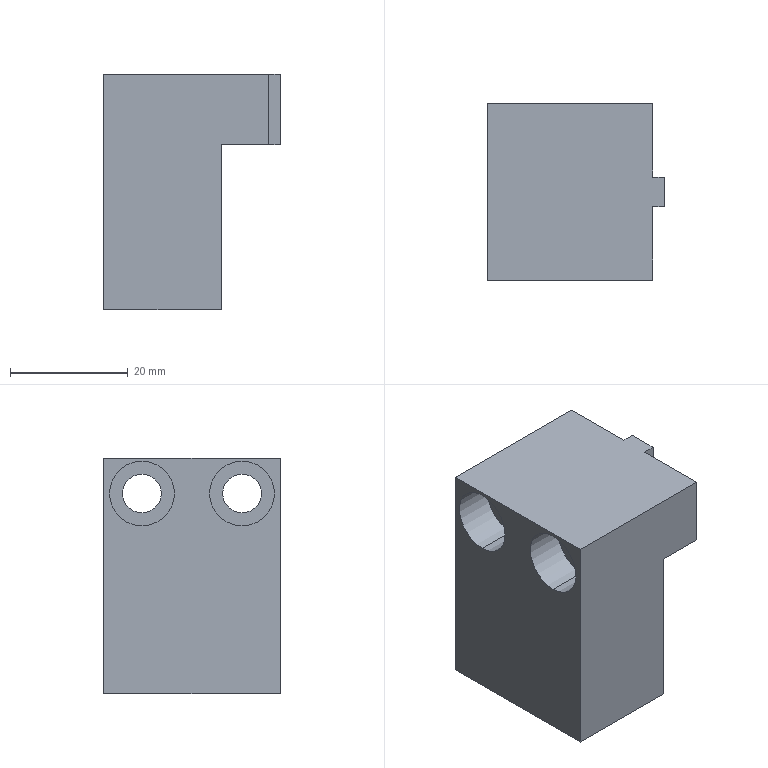Part | SolidWorks | features BaseBody 1 | 1 solid | 22 faces | box 30 x 30 x 40 mm | volume 24257 mm3 | plane 14 | cylinder 8 | commonest cylinder face diameters 6.6 x4 11 x4
STEP:
#1=CARTESIAN_POINT('',(-13.2,23.5,-11.5));
#2=VERTEX_POINT('',#1);
#3=CARTESIAN_POINT('',(-20.,23.5,-11.5));
#4=VERTEX_POINT('',#3);
#5=CARTESIAN_POINT('',(-20.,23.5,-11.5));
#6=DIRECTION('',(-1.,0.,0.));
#7=VECTOR('',#6,1000.);
#8=LINE('',#5,#7);
#9=EDGE_CURVE('',#2,#4,#8,.T.);
#10=ORIENTED_EDGE('',*,*,#9,.F.);
#11=CARTESIAN_POINT('',(-13.2,23.5,-0.5));
#12=VERTEX_POINT('',#11);
#13=CARTESIAN_POINT('',(-13.2,23.5,-6.));
#14=DIRECTION('',(-1.,0.,0.));
#15=DIRECTION('',(0.,0.,1.));
#16=AXIS2_PLACEMENT_3D('',#13,#14,#15);
#17=CIRCLE('',#16,5.5);
#18=EDGE_CURVE('',#12,#2,#17,.T.);
#19=ORIENTED_EDGE('',*,*,#18,.F.);
#20=CARTESIAN_POINT('',(-20.,23.5,-0.5));
#21=VERTEX_POINT('',#20);
#22=CARTESIAN_POINT('',(-20.,23.5,-0.5));
#23=DIRECTION('',(-1.,0.,0.));
#24=VECTOR('',#23,1000.);
#25=LINE('',#22,#24);
#26=EDGE_CURVE('',#12,#21,#25,.T.);
#27=ORIENTED_EDGE('',*,*,#26,.T.);
#28=CARTESIAN_POINT('',(-20.,23.5,-6.));
#29=DIRECTION('',(-1.,0.,0.));
#30=DIRECTION('',(0.,0.,1.));
#31=AXIS2_PLACEMENT_3D('',#28,#29,#30);
#32=CIRCLE('',#31,5.5);
#33=EDGE_CURVE('',#21,#4,#32,.T.);
#34=ORIENTED_EDGE('',*,*,#33,.T.);
#35=EDGE_LOOP('',(#10,#19,#27,#34));
#36=FACE_OUTER_BOUND('',#35,.T.);
#37=CARTESIAN_POINT('',(-20.,23.5,-6.));
#38=DIRECTION('',(-1.,0.,0.));
#39=DIRECTION('',(0.,0.,1.));
#40=AXIS2_PLACEMENT_3D('',#37,#38,#39);
#41=CYLINDRICAL_SURFACE('',#40,5.5);
#42=ADVANCED_FACE('',(#36),#41,.F.);
#43=CARTESIAN_POINT('',(-13.2,23.5,-2.7));
#44=VERTEX_POINT('',#43);
#45=CARTESIAN_POINT('',(-13.2,23.5,-9.3));
#46=VERTEX_POINT('',#45);
#47=CARTESIAN_POINT('',(-13.2,23.5,-6.));
#48=DIRECTION('',(-1.,0.,0.));
#49=DIRECTION('',(0.,0.,1.));
#50=AXIS2_PLACEMENT_3D('',#47,#48,#49);
#51=CIRCLE('',#50,3.3);
#52=EDGE_CURVE('',#44,#46,#51,.T.);
#53=ORIENTED_EDGE('',*,*,#52,.F.);
#54=CARTESIAN_POINT('',(-13.2,23.5,-6.));
#55=DIRECTION('',(-1.,0.,0.));
#56=DIRECTION('',(0.,0.,1.));
#57=AXIS2_PLACEMENT_3D('',#54,#55,#56);
#58=CIRCLE('',#57,3.3);
#59=EDGE_CURVE('',#46,#44,#58,.T.);
#60=ORIENTED_EDGE('',*,*,#59,.F.);
#61=EDGE_LOOP('',(#53,#60));
#62=FACE_BOUND('',#61,.T.);
#63=ORIENTED_EDGE('',*,*,#18,.T.);
#64=CARTESIAN_POINT('',(-13.2,23.5,-6.));
#65=DIRECTION('',(-1.,0.,0.));
#66=DIRECTION('',(0.,0.,1.));
#67=AXIS2_PLACEMENT_3D('',#64,#65,#66);
#68=CIRCLE('',#67,5.5);
#69=EDGE_CURVE('',#2,#12,#68,.T.);
#70=ORIENTED_EDGE('',*,*,#69,.T.);
#71=EDGE_LOOP('',(#63,#70));
#72=FACE_OUTER_BOUND('',#71,.T.);
#73=CARTESIAN_POINT('',(-13.2,26.8,-6.));
#74=DIRECTION('',(1.,0.,0.));
#75=DIRECTION('',(0.,0.,-1.));
#76=AXIS2_PLACEMENT_3D('',#73,#74,#75);
#77=PLANE('',#76);
#78=ADVANCED_FACE('',(#62,#72),#77,.F.);
#79=CARTESIAN_POINT('',(8.,23.5,-9.3));
#80=VERTEX_POINT('',#79);
#81=CARTESIAN_POINT('',(-20.,23.5,-9.3));
#82=DIRECTION('',(-1.,0.,0.));
#83=VECTOR('',#82,1000.);
#84=LINE('',#81,#83);
#85=EDGE_CURVE('',#80,#46,#84,.T.);
#86=ORIENTED_EDGE('',*,*,#85,.F.);
#87=CARTESIAN_POINT('',(8.,23.5,-2.7));
#88=VERTEX_POINT('',#87);
#89=CARTESIAN_POINT('',(8.,23.5,-6.));
#90=DIRECTION('',(1.,0.,0.));
#91=DIRECTION('',(0.,0.,-1.));
#92=AXIS2_PLACEMENT_3D('',#89,#90,#91);
#93=CIRCLE('',#92,3.3);
#94=EDGE_CURVE('',#80,#88,#93,.T.);
#95=ORIENTED_EDGE('',*,*,#94,.T.);
#96=CARTESIAN_POINT('',(-20.,23.5,-2.7));
#97=DIRECTION('',(-1.,0.,0.));
#98=VECTOR('',#97,1000.);
#99=LINE('',#96,#98);
#100=EDGE_CURVE('',#88,#44,#99,.T.);
#101=ORIENTED_EDGE('',*,*,#100,.T.);
#102=ORIENTED_EDGE('',*,*,#52,.T.);
#103=EDGE_LOOP('',(#86,#95,#101,#102));
#104=FACE_OUTER_BOUND('',#103,.T.);
#105=CARTESIAN_POINT('',(-20.,23.5,-6.));
#106=DIRECTION('',(-1.,0.,0.));
#107=DIRECTION('',(0.,0.,1.));
#108=AXIS2_PLACEMENT_3D('',#105,#106,#107);
#109=CYLINDRICAL_SURFACE('',#108,3.3);
#110=ADVANCED_FACE('',(#104),#109,.F.);
#111=CARTESIAN_POINT('',(-13.2,6.5,-11.5));
#112=VERTEX_POINT('',#111);
#113=CARTESIAN_POINT('',(-20.,6.5,-11.5));
#114=VERTEX_POINT('',#113);
#115=CARTESIAN_POINT('',(-20.,6.5,-11.5));
#116=DIRECTION('',(-1.,0.,0.));
#117=VECTOR('',#116,1000.);
#118=LINE('',#115,#117);
#119=EDGE_CURVE('',#112,#114,#118,.T.);
#120=ORIENTED_EDGE('',*,*,#119,.F.);
#121=CARTESIAN_POINT('',(-13.2,6.5,-0.5));
#122=VERTEX_POINT('',#121);
#123=CARTESIAN_POINT('',(-13.2,6.5,-6.));
#124=DIRECTION('',(-1.,0.,0.));
#125=DIRECTION('',(0.,0.,1.));
#126=AXIS2_PLACEMENT_3D('',#123,#124,#125);
#127=CIRCLE('',#126,5.5);
#128=EDGE_CURVE('',#122,#112,#127,.T.);
#129=ORIENTED_EDGE('',*,*,#128,.F.);
#130=CARTESIAN_POINT('',(-20.,6.5,-0.5));
#131=VERTEX_POINT('',#130);
#132=CARTESIAN_POINT('',(-20.,6.5,-0.5));
#133=DIRECTION('',(-1.,0.,0.));
#134=VECTOR('',#133,1000.);
#135=LINE('',#132,#134);
#136=EDGE_CURVE('',#122,#131,#135,.T.);
#137=ORIENTED_EDGE('',*,*,#136,.T.);
#138=CARTESIAN_POINT('',(-20.,6.5,-6.));
#139=DIRECTION('',(-1.,0.,0.));
#140=DIRECTION('',(0.,0.,1.));
#141=AXIS2_PLACEMENT_3D('',#138,#139,#140);
#142=CIRCLE('',#141,5.5);
#143=EDGE_CURVE('',#131,#114,#142,.T.);
#144=ORIENTED_EDGE('',*,*,#143,.T.);
#145=EDGE_LOOP('',(#120,#129,#137,#144));
#146=FACE_OUTER_BOUND('',#145,.T.);
#147=CARTESIAN_POINT('',(-20.,6.5,-6.));
#148=DIRECTION('',(-1.,0.,0.));
#149=DIRECTION('',(0.,0.,1.));
#150=AXIS2_PLACEMENT_3D('',#147,#148,#149);
#151=CYLINDRICAL_SURFACE('',#150,5.5);
#152=ADVANCED_FACE('',(#146),#151,.F.);
#153=CARTESIAN_POINT('',(-13.2,6.5,-2.7));
#154=VERTEX_POINT('',#153);
#155=CARTESIAN_POINT('',(-13.2,6.5,-9.3));
#156=VERTEX_POINT('',#155);
#157=CARTESIAN_POINT('',(-13.2,6.5,-6.));
#158=DIRECTION('',(-1.,0.,0.));
#159=DIRECTION('',(0.,0.,1.));
#160=AXIS2_PLACEMENT_3D('',#157,#158,#159);
#161=CIRCLE('',#160,3.3);
#162=EDGE_CURVE('',#154,#156,#161,.T.);
#163=ORIENTED_EDGE('',*,*,#162,.F.);
#164=CARTESIAN_POINT('',(-13.2,6.5,-6.));
#165=DIRECTION('',(-1.,0.,0.));
#166=DIRECTION('',(0.,0.,1.));
#167=AXIS2_PLACEMENT_3D('',#164,#165,#166);
#168=CIRCLE('',#167,3.3);
#169=EDGE_CURVE('',#156,#154,#168,.T.);
#170=ORIENTED_EDGE('',*,*,#169,.F.);
#171=EDGE_LOOP('',(#163,#170));
#172=FACE_BOUND('',#171,.T.);
#173=ORIENTED_EDGE('',*,*,#128,.T.);
#174=CARTESIAN_POINT('',(-13.2,6.5,-6.));
#175=DIRECTION('',(-1.,0.,0.));
#176=DIRECTION('',(0.,0.,1.));
#177=AXIS2_PLACEMENT_3D('',#174,#175,#176);
#178=CIRCLE('',#177,5.5);
#179=EDGE_CURVE('',#112,#122,#178,.T.);
#180=ORIENTED_EDGE('',*,*,#179,.T.);
#181=EDGE_LOOP('',(#173,#180));
#182=FACE_OUTER_BOUND('',#181,.T.);
#183=CARTESIAN_POINT('',(-13.2,9.8,-6.));
#184=DIRECTION('',(1.,0.,0.));
#185=DIRECTION('',(0.,0.,-1.));
#186=AXIS2_PLACEMENT_3D('',#183,#184,#185);
#187=PLANE('',#186);
#188=ADVANCED_FACE('',(#172,#182),#187,.F.);
#189=CARTESIAN_POINT('',(8.,6.5,-9.3));
#190=VERTEX_POINT('',#189);
#191=CARTESIAN_POINT('',(-20.,6.5,-9.3));
#192=DIRECTION('',(-1.,0.,0.));
#193=VECTOR('',#192,1000.);
#194=LINE('',#191,#193);
#195=EDGE_CURVE('',#190,#156,#194,.T.);
#196=ORIENTED_EDGE('',*,*,#195,.F.);
#197=CARTESIAN_POINT('',(8.,6.5,-2.7));
#198=VERTEX_POINT('',#197);
#199=CARTESIAN_POINT('',(8.,6.5,-6.));
#200=DIRECTION('',(1.,0.,0.));
#201=DIRECTION('',(0.,0.,-1.));
#202=AXIS2_PLACEMENT_3D('',#199,#200,#201);
#203=CIRCLE('',#202,3.3);
#204=EDGE_CURVE('',#190,#198,#203,.T.);
#205=ORIENTED_EDGE('',*,*,#204,.T.);
#206=CARTESIAN_POINT('',(-20.,6.5,-2.7));
#207=DIRECTION('',(-1.,0.,0.));
#208=VECTOR('',#207,1000.);
#209=LINE('',#206,#208);
#210=EDGE_CURVE('',#198,#154,#209,.T.);
#211=ORIENTED_EDGE('',*,*,#210,.T.);
#212=ORIENTED_EDGE('',*,*,#162,.T.);
#213=EDGE_LOOP('',(#196,#205,#211,#212));
#214=FACE_OUTER_BOUND('',#213,.T.);
#215=CARTESIAN_POINT('',(-20.,6.5,-6.));
#216=DIRECTION('',(-1.,0.,0.));
#217=DIRECTION('',(0.,0.,1.));
#218=AXIS2_PLACEMENT_3D('',#215,#216,#217);
#219=CYLINDRICAL_SURFACE('',#218,3.3);
#220=ADVANCED_FACE('',(#214),#219,.F.);
#221=CARTESIAN_POINT('',(8.,23.5,-6.));
#222=DIRECTION('',(1.,0.,0.));
#223=DIRECTION('',(0.,0.,-1.));
#224=AXIS2_PLACEMENT_3D('',#221,#222,#223);
#225=CIRCLE('',#224,3.3);
#226=EDGE_CURVE('',#88,#80,#225,.T.);
#227=ORIENTED_EDGE('',*,*,#226,.F.);
#228=ORIENTED_EDGE('',*,*,#94,.F.);
#229=EDGE_LOOP('',(#227,#228));
#230=FACE_BOUND('',#229,.T.);
#231=CARTESIAN_POINT('',(8.,30.,0.));
#232=VERTEX_POINT('',#231);
#233=CARTESIAN_POINT('',(8.,17.5,0.));
#234=VERTEX_POINT('',#233);
#235=CARTESIAN_POINT('',(8.,30.,0.));
#236=DIRECTION('',(0.,-1.,0.));
#237=VECTOR('',#236,1000.);
#238=LINE('',#235,#237);
#239=EDGE_CURVE('',#232,#234,#238,.T.);
#240=ORIENTED_EDGE('',*,*,#239,.T.);
#241=CARTESIAN_POINT('',(8.,17.5,-12.));
#242=VERTEX_POINT('',#241);
#243=CARTESIAN_POINT('',(8.,17.5,0.));
#244=DIRECTION('',(0.,0.,-1.));
#245=VECTOR('',#244,1000.);
#246=LINE('',#243,#245);
#247=EDGE_CURVE('',#234,#242,#246,.T.);
#248=ORIENTED_EDGE('',*,*,#247,.T.);
#249=CARTESIAN_POINT('',(8.,30.,-12.));
#250=VERTEX_POINT('',#249);
#251=CARTESIAN_POINT('',(8.,30.,-12.));
#252=DIRECTION('',(0.,1.,0.));
#253=VECTOR('',#252,1000.);
#254=LINE('',#251,#253);
#255=EDGE_CURVE('',#242,#250,#254,.T.);
#256=ORIENTED_EDGE('',*,*,#255,.T.);
#257=CARTESIAN_POINT('',(8.,30.,0.));
#258=DIRECTION('',(0.,0.,1.));
#259=VECTOR('',#258,1000.);
#260=LINE('',#257,#259);
#261=EDGE_CURVE('',#250,#232,#260,.T.);
#262=ORIENTED_EDGE('',*,*,#261,.T.);
#263=EDGE_LOOP('',(#240,#248,#256,#262));
#264=FACE_OUTER_BOUND('',#263,.T.);
#265=CARTESIAN_POINT('',(8.,0.,0.));
#266=DIRECTION('',(1.,0.,0.));
#267=DIRECTION('',(0.,1.,0.));
#268=AXIS2_PLACEMENT_3D('',#265,#266,#267);
#269=PLANE('',#268);
#270=ADVANCED_FACE('',(#230,#264),#269,.T.);
#271=CARTESIAN_POINT('',(10.,17.5,0.));
#272=VERTEX_POINT('',#271);
#273=CARTESIAN_POINT('',(10.,17.5,-12.));
#274=VERTEX_POINT('',#273);
#275=CARTESIAN_POINT('',(10.,17.5,0.));
#276=DIRECTION('',(0.,0.,-1.));
#277=VECTOR('',#276,1000.);
#278=LINE('',#275,#277);
#279=EDGE_CURVE('',#272,#274,#278,.T.);
#280=ORIENTED_EDGE('',*,*,#279,.T.);
#281=CARTESIAN_POINT('',(8.,17.5,-12.));
#282=DIRECTION('',(1.,0.,0.));
#283=VECTOR('',#282,1000.);
#284=LINE('',#281,#283);
#285=EDGE_CURVE('',#242,#274,#284,.T.);
#286=ORIENTED_EDGE('',*,*,#285,.F.);
#287=ORIENTED_EDGE('',*,*,#247,.F.);
#288=CARTESIAN_POINT('',(8.,17.5,0.));
#289=DIRECTION('',(1.,0.,0.));
#290=VECTOR('',#289,1000.);
#291=LINE('',#288,#290);
#292=EDGE_CURVE('',#234,#272,#291,.T.);
#293=ORIENTED_EDGE('',*,*,#292,.T.);
#294=EDGE_LOOP('',(#280,#286,#287,#293));
#295=FACE_OUTER_BOUND('',#294,.T.);
#296=CARTESIAN_POINT('',(8.,17.5,0.));
#297=DIRECTION('',(0.,-1.,0.));
#298=DIRECTION('',(0.,0.,-1.));
#299=AXIS2_PLACEMENT_3D('',#296,#297,#298);
#300=PLANE('',#299);
#301=ADVANCED_FACE('',(#295),#300,.F.);
#302=CARTESIAN_POINT('',(8.,6.5,-6.));
#303=DIRECTION('',(1.,0.,0.));
#304=DIRECTION('',(0.,0.,-1.));
#305=AXIS2_PLACEMENT_3D('',#302,#303,#304);
#306=CIRCLE('',#305,3.3);
#307=EDGE_CURVE('',#198,#190,#306,.T.);
#308=ORIENTED_EDGE('',*,*,#307,.F.);
#309=ORIENTED_EDGE('',*,*,#204,.F.);
#310=EDGE_LOOP('',(#308,#309));
#311=FACE_BOUND('',#310,.T.);
#312=CARTESIAN_POINT('',(8.,0.,0.));
#313=VERTEX_POINT('',#312);
#314=CARTESIAN_POINT('',(8.,0.,-12.));
#315=VERTEX_POINT('',#314);
#316=CARTESIAN_POINT('',(8.,0.,0.));
#317=DIRECTION('',(0.,0.,-1.));
#318=VECTOR('',#317,1000.);
#319=LINE('',#316,#318);
#320=EDGE_CURVE('',#313,#315,#319,.T.);
#321=ORIENTED_EDGE('',*,*,#320,.T.);
#322=CARTESIAN_POINT('',(8.,12.5,-12.));
#323=VERTEX_POINT('',#322);
#324=CARTESIAN_POINT('',(8.,0.,-12.));
#325=DIRECTION('',(0.,1.,0.));
#326=VECTOR('',#325,1000.);
#327=LINE('',#324,#326);
#328=EDGE_CURVE('',#315,#323,#327,.T.);
#329=ORIENTED_EDGE('',*,*,#328,.T.);
#330=CARTESIAN_POINT('',(8.,12.5,0.));
#331=VERTEX_POINT('',#330);
#332=CARTESIAN_POINT('',(8.,12.5,0.));
#333=DIRECTION('',(0.,0.,1.));
#334=VECTOR('',#333,1000.);
#335=LINE('',#332,#334);
#336=EDGE_CURVE('',#323,#331,#335,.T.);
#337=ORIENTED_EDGE('',*,*,#336,.T.);
#338=CARTESIAN_POINT('',(8.,0.,0.));
#339=DIRECTION('',(0.,-1.,0.));
#340=VECTOR('',#339,1000.);
#341=LINE('',#338,#340);
#342=EDGE_CURVE('',#331,#313,#341,.T.);
#343=ORIENTED_EDGE('',*,*,#342,.T.);
#344=EDGE_LOOP('',(#321,#329,#337,#343));
#345=FACE_OUTER_BOUND('',#344,.T.);
#346=CARTESIAN_POINT('',(8.,0.,0.));
#347=DIRECTION('',(1.,0.,0.));
#348=DIRECTION('',(0.,1.,0.));
#349=AXIS2_PLACEMENT_3D('',#346,#347,#348);
#350=PLANE('',#349);
#351=ADVANCED_FACE('',(#311,#345),#350,.T.);
#352=CARTESIAN_POINT('',(10.,12.5,-12.));
#353=VERTEX_POINT('',#352);
#354=CARTESIAN_POINT('',(10.,12.5,0.));
#355=VERTEX_POINT('',#354);
#356=CARTESIAN_POINT('',(10.,12.5,0.));
#357=DIRECTION('',(0.,0.,1.));
#358=VECTOR('',#357,1000.);
#359=LINE('',#356,#358);
#360=EDGE_CURVE('',#353,#355,#359,.T.);
#361=ORIENTED_EDGE('',*,*,#360,.T.);
#362=CARTESIAN_POINT('',(8.,12.5,0.));
#363=DIRECTION('',(1.,0.,0.));
#364=VECTOR('',#363,1000.);
#365=LINE('',#362,#364);
#366=EDGE_CURVE('',#331,#355,#365,.T.);
#367=ORIENTED_EDGE('',*,*,#366,.F.);
#368=ORIENTED_EDGE('',*,*,#336,.F.);
#369=CARTESIAN_POINT('',(8.,12.5,-12.));
#370=DIRECTION('',(1.,0.,0.));
#371=VECTOR('',#370,1000.);
#372=LINE('',#369,#371);
#373=EDGE_CURVE('',#323,#353,#372,.T.);
#374=ORIENTED_EDGE('',*,*,#373,.T.);
#375=EDGE_LOOP('',(#361,#367,#368,#374));
#376=FACE_OUTER_BOUND('',#375,.T.);
#377=CARTESIAN_POINT('',(8.,12.5,0.));
#378=DIRECTION('',(0.,1.,0.));
#379=DIRECTION('',(0.,0.,-1.));
#380=AXIS2_PLACEMENT_3D('',#377,#378,#379);
#381=PLANE('',#380);
#382=ADVANCED_FACE('',(#376),#381,.F.);
#383=CARTESIAN_POINT('',(10.,30.,0.));
#384=DIRECTION('',(0.,-1.,0.));
#385=VECTOR('',#384,1000.);
#386=LINE('',#383,#385);
#387=EDGE_CURVE('',#272,#355,#386,.T.);
#388=ORIENTED_EDGE('',*,*,#387,.F.);
#389=ORIENTED_EDGE('',*,*,#292,.F.);
#390=ORIENTED_EDGE('',*,*,#239,.F.);
#391=CARTESIAN_POINT('',(-20.,30.,0.));
#392=VERTEX_POINT('',#391);
#393=CARTESIAN_POINT('',(-20.,30.,0.));
#394=DIRECTION('',(1.,0.,0.));
#395=VECTOR('',#394,1000.);
#396=LINE('',#393,#395);
#397=EDGE_CURVE('',#392,#232,#396,.T.);
#398=ORIENTED_EDGE('',*,*,#397,.F.);
#399=CARTESIAN_POINT('',(-20.,0.,0.));
#400=VERTEX_POINT('',#399);
#401=CARTESIAN_POINT('',(-20.,30.,0.));
#402=DIRECTION('',(0.,-1.,0.));
#403=VECTOR('',#402,1000.);
#404=LINE('',#401,#403);
#405=EDGE_CURVE('',#392,#400,#404,.T.);
#406=ORIENTED_EDGE('',*,*,#405,.T.);
#407=CARTESIAN_POINT('',(-20.,0.,0.));
#408=DIRECTION('',(1.,0.,0.));
#409=VECTOR('',#408,1000.);
#410=LINE('',#407,#409);
#411=EDGE_CURVE('',#400,#313,#410,.T.);
#412=ORIENTED_EDGE('',*,*,#411,.T.);
#413=ORIENTED_EDGE('',*,*,#342,.F.);
#414=ORIENTED_EDGE('',*,*,#366,.T.);
#415=EDGE_LOOP('',(#388,#389,#390,#398,#406,#412,#413,#414));
#416=FACE_OUTER_BOUND('',#415,.T.);
#417=CARTESIAN_POINT('',(-20.,30.,0.));
#418=DIRECTION('',(0.,0.,-1.));
#419=DIRECTION('',(0.,-1.,0.));
#420=AXIS2_PLACEMENT_3D('',#417,#418,#419);
#421=PLANE('',#420);
#422=ADVANCED_FACE('',(#416),#421,.F.);
#423=CARTESIAN_POINT('',(0.,0.,-40.));
#424=VERTEX_POINT('',#423);
#425=CARTESIAN_POINT('',(-20.,0.,-40.));
#426=VERTEX_POINT('',#425);
#427=CARTESIAN_POINT('',(0.,0.,-40.));
#428=DIRECTION('',(-1.,0.,0.));
#429=VECTOR('',#428,1000.);
#430=LINE('',#427,#429);
#431=EDGE_CURVE('',#424,#426,#430,.T.);
#432=ORIENTED_EDGE('',*,*,#431,.T.);
#433=CARTESIAN_POINT('',(-20.,30.,-40.));
#434=VERTEX_POINT('',#433);
#435=CARTESIAN_POINT('',(-20.,30.,-40.));
#436=DIRECTION('',(0.,-1.,0.));
#437=VECTOR('',#436,1000.);
#438=LINE('',#435,#437);
#439=EDGE_CURVE('',#434,#426,#438,.T.);
#440=ORIENTED_EDGE('',*,*,#439,.F.);
#441=CARTESIAN_POINT('',(0.,30.,-40.));
#442=VERTEX_POINT('',#441);
#443=CARTESIAN_POINT('',(0.,30.,-40.));
#444=DIRECTION('',(-1.,0.,0.));
#445=VECTOR('',#444,1000.);
#446=LINE('',#443,#445);
#447=EDGE_CURVE('',#442,#434,#446,.T.);
#448=ORIENTED_EDGE('',*,*,#447,.F.);
#449=CARTESIAN_POINT('',(0.,30.,-40.));
#450=DIRECTION('',(0.,-1.,0.));
#451=VECTOR('',#450,1000.);
#452=LINE('',#449,#451);
#453=EDGE_CURVE('',#442,#424,#452,.T.);
#454=ORIENTED_EDGE('',*,*,#453,.T.);
#455=EDGE_LOOP('',(#432,#440,#448,#454));
#456=FACE_OUTER_BOUND('',#455,.T.);
#457=CARTESIAN_POINT('',(0.,30.,-40.));
#458=DIRECTION('',(0.,0.,1.));
#459=DIRECTION('',(1.,0.,0.));
#460=AXIS2_PLACEMENT_3D('',#457,#458,#459);
#461=PLANE('',#460);
#462=ADVANCED_FACE('',(#456),#461,.F.);
#463=CARTESIAN_POINT('',(0.,0.,-12.));
#464=VERTEX_POINT('',#463);
#465=CARTESIAN_POINT('',(0.,0.,-12.));
#466=DIRECTION('',(0.,0.,-1.));
#467=VECTOR('',#466,1000.);
#468=LINE('',#465,#467);
#469=EDGE_CURVE('',#464,#424,#468,.T.);
#470=ORIENTED_EDGE('',*,*,#469,.T.);
#471=ORIENTED_EDGE('',*,*,#453,.F.);
#472=CARTESIAN_POINT('',(0.,30.,-12.));
#473=VERTEX_POINT('',#472);
#474=CARTESIAN_POINT('',(0.,30.,-12.));
#475=DIRECTION('',(0.,0.,-1.));
#476=VECTOR('',#475,1000.);
#477=LINE('',#474,#476);
#478=EDGE_CURVE('',#473,#442,#477,.T.);
#479=ORIENTED_EDGE('',*,*,#478,.F.);
#480=CARTESIAN_POINT('',(0.,30.,-12.));
#481=DIRECTION('',(0.,-1.,0.));
#482=VECTOR('',#481,1000.);
#483=LINE('',#480,#482);
#484=EDGE_CURVE('',#473,#464,#483,.T.);
#485=ORIENTED_EDGE('',*,*,#484,.T.);
#486=EDGE_LOOP('',(#470,#471,#479,#485));
#487=FACE_OUTER_BOUND('',#486,.T.);
#488=CARTESIAN_POINT('',(0.,30.,-12.));
#489=DIRECTION('',(-1.,0.,0.));
#490=DIRECTION('',(0.,0.,1.));
#491=AXIS2_PLACEMENT_3D('',#488,#489,#490);
#492=PLANE('',#491);
#493=ADVANCED_FACE('',(#487),#492,.F.);
#494=ORIENTED_EDGE('',*,*,#255,.F.);
#495=ORIENTED_EDGE('',*,*,#285,.T.);
#496=CARTESIAN_POINT('',(10.,30.,-12.));
#497=DIRECTION('',(0.,-1.,0.));
#498=VECTOR('',#497,1000.);
#499=LINE('',#496,#498);
#500=EDGE_CURVE('',#274,#353,#499,.T.);
#501=ORIENTED_EDGE('',*,*,#500,.T.);
#502=ORIENTED_EDGE('',*,*,#373,.F.);
#503=ORIENTED_EDGE('',*,*,#328,.F.);
#504=CARTESIAN_POINT('',(10.,0.,-12.));
#505=DIRECTION('',(-1.,0.,0.));
#506=VECTOR('',#505,1000.);
#507=LINE('',#504,#506);
#508=EDGE_CURVE('',#315,#464,#507,.T.);
#509=ORIENTED_EDGE('',*,*,#508,.T.);
#510=ORIENTED_EDGE('',*,*,#484,.F.);
#511=CARTESIAN_POINT('',(10.,30.,-12.));
#512=DIRECTION('',(-1.,0.,0.));
#513=VECTOR('',#512,1000.);
#514=LINE('',#511,#513);
#515=EDGE_CURVE('',#250,#473,#514,.T.);
#516=ORIENTED_EDGE('',*,*,#515,.F.);
#517=EDGE_LOOP('',(#494,#495,#501,#502,#503,#509,#510,#516));
#518=FACE_OUTER_BOUND('',#517,.T.);
#519=CARTESIAN_POINT('',(10.,30.,-12.));
#520=DIRECTION('',(0.,0.,1.));
#521=DIRECTION('',(1.,0.,0.));
#522=AXIS2_PLACEMENT_3D('',#519,#520,#521);
#523=PLANE('',#522);
#524=ADVANCED_FACE('',(#518),#523,.F.);
#525=ORIENTED_EDGE('',*,*,#500,.F.);
#526=ORIENTED_EDGE('',*,*,#279,.F.);
#527=ORIENTED_EDGE('',*,*,#387,.T.);
#528=ORIENTED_EDGE('',*,*,#360,.F.);
#529=EDGE_LOOP('',(#525,#526,#527,#528));
#530=FACE_OUTER_BOUND('',#529,.T.);
#531=CARTESIAN_POINT('',(10.,30.,0.));
#532=DIRECTION('',(-1.,0.,0.));
#533=DIRECTION('',(0.,0.,1.));
#534=AXIS2_PLACEMENT_3D('',#531,#532,#533);
#535=PLANE('',#534);
#536=ADVANCED_FACE('',(#530),#535,.F.);
#537=ORIENTED_EDGE('',*,*,#320,.F.);
#538=ORIENTED_EDGE('',*,*,#411,.F.);
#539=CARTESIAN_POINT('',(-20.,0.,-40.));
#540=DIRECTION('',(0.,0.,1.));
#541=VECTOR('',#540,1000.);
#542=LINE('',#539,#541);
#543=EDGE_CURVE('',#426,#400,#542,.T.);
#544=ORIENTED_EDGE('',*,*,#543,.F.);
#545=ORIENTED_EDGE('',*,*,#431,.F.);
#546=ORIENTED_EDGE('',*,*,#469,.F.);
#547=ORIENTED_EDGE('',*,*,#508,.F.);
#548=EDGE_LOOP('',(#537,#538,#544,#545,#546,#547));
#549=FACE_OUTER_BOUND('',#548,.T.);
#550=CARTESIAN_POINT('',(0.,0.,0.));
#551=DIRECTION('',(0.,1.,0.));
#552=DIRECTION('',(1.,0.,0.));
#553=AXIS2_PLACEMENT_3D('',#550,#551,#552);
#554=PLANE('',#553);
#555=ADVANCED_FACE('',(#549),#554,.F.);
#556=ORIENTED_EDGE('',*,*,#397,.T.);
#557=ORIENTED_EDGE('',*,*,#261,.F.);
#558=ORIENTED_EDGE('',*,*,#515,.T.);
#559=ORIENTED_EDGE('',*,*,#478,.T.);
#560=ORIENTED_EDGE('',*,*,#447,.T.);
#561=CARTESIAN_POINT('',(-20.,30.,-40.));
#562=DIRECTION('',(0.,0.,1.));
#563=VECTOR('',#562,1000.);
#564=LINE('',#561,#563);
#565=EDGE_CURVE('',#434,#392,#564,.T.);
#566=ORIENTED_EDGE('',*,*,#565,.T.);
#567=EDGE_LOOP('',(#556,#557,#558,#559,#560,#566));
#568=FACE_OUTER_BOUND('',#567,.T.);
#569=CARTESIAN_POINT('',(0.,30.,0.));
#570=DIRECTION('',(0.,1.,0.));
#571=DIRECTION('',(1.,0.,0.));
#572=AXIS2_PLACEMENT_3D('',#569,#570,#571);
#573=PLANE('',#572);
#574=ADVANCED_FACE('',(#568),#573,.T.);
#575=ORIENTED_EDGE('',*,*,#33,.F.);
#576=CARTESIAN_POINT('',(-20.,23.5,-6.));
#577=DIRECTION('',(-1.,0.,0.));
#578=DIRECTION('',(0.,0.,1.));
#579=AXIS2_PLACEMENT_3D('',#576,#577,#578);
#580=CIRCLE('',#579,5.5);
#581=EDGE_CURVE('',#4,#21,#580,.T.);
#582=ORIENTED_EDGE('',*,*,#581,.F.);
#583=EDGE_LOOP('',(#575,#582));
#584=FACE_BOUND('',#583,.T.);
#585=ORIENTED_EDGE('',*,*,#143,.F.);
#586=CARTESIAN_POINT('',(-20.,6.5,-6.));
#587=DIRECTION('',(-1.,0.,0.));
#588=DIRECTION('',(0.,0.,1.));
#589=AXIS2_PLACEMENT_3D('',#586,#587,#588);
#590=CIRCLE('',#589,5.5);
#591=EDGE_CURVE('',#114,#131,#590,.T.);
#592=ORIENTED_EDGE('',*,*,#591,.F.);
#593=EDGE_LOOP('',(#585,#592));
#594=FACE_BOUND('',#593,.T.);
#595=ORIENTED_EDGE('',*,*,#543,.T.);
#596=ORIENTED_EDGE('',*,*,#405,.F.);
#597=ORIENTED_EDGE('',*,*,#565,.F.);
#598=ORIENTED_EDGE('',*,*,#439,.T.);
#599=EDGE_LOOP('',(#595,#596,#597,#598));
#600=FACE_OUTER_BOUND('',#599,.T.);
#601=CARTESIAN_POINT('',(-20.,30.,-40.));
#602=DIRECTION('',(1.,0.,0.));
#603=DIRECTION('',(0.,0.,-1.));
#604=AXIS2_PLACEMENT_3D('',#601,#602,#603);
#605=PLANE('',#604);
#606=ADVANCED_FACE('',(#584,#594,#600),#605,.F.);
#607=ORIENTED_EDGE('',*,*,#307,.T.);
#608=ORIENTED_EDGE('',*,*,#195,.T.);
#609=ORIENTED_EDGE('',*,*,#169,.T.);
#610=ORIENTED_EDGE('',*,*,#210,.F.);
#611=EDGE_LOOP('',(#607,#608,#609,#610));
#612=FACE_OUTER_BOUND('',#611,.T.);
#613=CARTESIAN_POINT('',(-20.,6.5,-6.));
#614=DIRECTION('',(-1.,0.,0.));
#615=DIRECTION('',(0.,0.,1.));
#616=AXIS2_PLACEMENT_3D('',#613,#614,#615);
#617=CYLINDRICAL_SURFACE('',#616,3.3);
#618=ADVANCED_FACE('',(#612),#617,.F.);
#619=ORIENTED_EDGE('',*,*,#179,.F.);
#620=ORIENTED_EDGE('',*,*,#119,.T.);
#621=ORIENTED_EDGE('',*,*,#591,.T.);
#622=ORIENTED_EDGE('',*,*,#136,.F.);
#623=EDGE_LOOP('',(#619,#620,#621,#622));
#624=FACE_OUTER_BOUND('',#623,.T.);
#625=CARTESIAN_POINT('',(-20.,6.5,-6.));
#626=DIRECTION('',(-1.,0.,0.));
#627=DIRECTION('',(0.,0.,1.));
#628=AXIS2_PLACEMENT_3D('',#625,#626,#627);
#629=CYLINDRICAL_SURFACE('',#628,5.5);
#630=ADVANCED_FACE('',(#624),#629,.F.);
#631=ORIENTED_EDGE('',*,*,#226,.T.);
#632=ORIENTED_EDGE('',*,*,#85,.T.);
#633=ORIENTED_EDGE('',*,*,#59,.T.);
#634=ORIENTED_EDGE('',*,*,#100,.F.);
#635=EDGE_LOOP('',(#631,#632,#633,#634));
#636=FACE_OUTER_BOUND('',#635,.T.);
#637=CARTESIAN_POINT('',(-20.,23.5,-6.));
#638=DIRECTION('',(-1.,0.,0.));
#639=DIRECTION('',(0.,0.,1.));
#640=AXIS2_PLACEMENT_3D('',#637,#638,#639);
#641=CYLINDRICAL_SURFACE('',#640,3.3);
#642=ADVANCED_FACE('',(#636),#641,.F.);
#643=ORIENTED_EDGE('',*,*,#69,.F.);
#644=ORIENTED_EDGE('',*,*,#9,.T.);
#645=ORIENTED_EDGE('',*,*,#581,.T.);
#646=ORIENTED_EDGE('',*,*,#26,.F.);
#647=EDGE_LOOP('',(#643,#644,#645,#646));
#648=FACE_OUTER_BOUND('',#647,.T.);
#649=CARTESIAN_POINT('',(-20.,23.5,-6.));
#650=DIRECTION('',(-1.,0.,0.));
#651=DIRECTION('',(0.,0.,1.));
#652=AXIS2_PLACEMENT_3D('',#649,#650,#651);
#653=CYLINDRICAL_SURFACE('',#652,5.5);
#654=ADVANCED_FACE('',(#648),#653,.F.);
#655=CLOSED_SHELL('',(#42,#78,#110,#152,#188,#220,#270,#301,#351,#382,#422,#462,#493,#524,#536,#555,#574,#606,#618,#630,#642,#654));
#656=MANIFOLD_SOLID_BREP('',#655);
#657=CARTESIAN_POINT('',(0.,0.,0.));
#658=DIRECTION('',(0.,0.,1.));
#659=DIRECTION('',(1.,0.,0.));
#660=AXIS2_PLACEMENT_3D('',#657,#658,#659);
#661=(LENGTH_UNIT()NAMED_UNIT(*)SI_UNIT(.MILLI.,.METRE.));
#662=UNCERTAINTY_MEASURE_WITH_UNIT(LENGTH_MEASURE(0.00001),#661,'','');
#663=(NAMED_UNIT(*)PLANE_ANGLE_UNIT()SI_UNIT($,.RADIAN.));
#664=(NAMED_UNIT(*)SI_UNIT($,.STERADIAN.)SOLID_ANGLE_UNIT());
#665=(GEOMETRIC_REPRESENTATION_CONTEXT(3)GLOBAL_UNCERTAINTY_ASSIGNED_CONTEXT((#662))GLOBAL_UNIT_ASSIGNED_CONTEXT((#661,#663,#664))REPRESENTATION_CONTEXT('',''));
#666=ADVANCED_BREP_SHAPE_REPRESENTATION('',(#656,#660),#665);